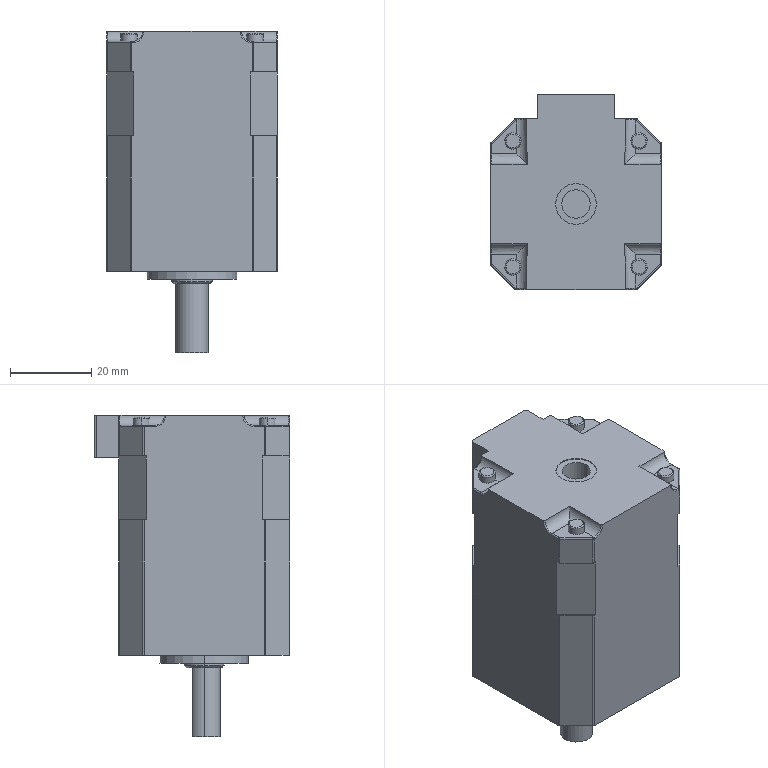Part | NX | features BREP 1 | 1 solid | 171 faces | box 42 x 48 x 79 mm | volume 100479 mm3 | cylinder 75 | plane 70 | torus 20 | spline 4 | cone 2 | commonest cylinder face diameters 1 x18 0.6 x12 1.118 x10 3.2 x8 4 x8 5 x8